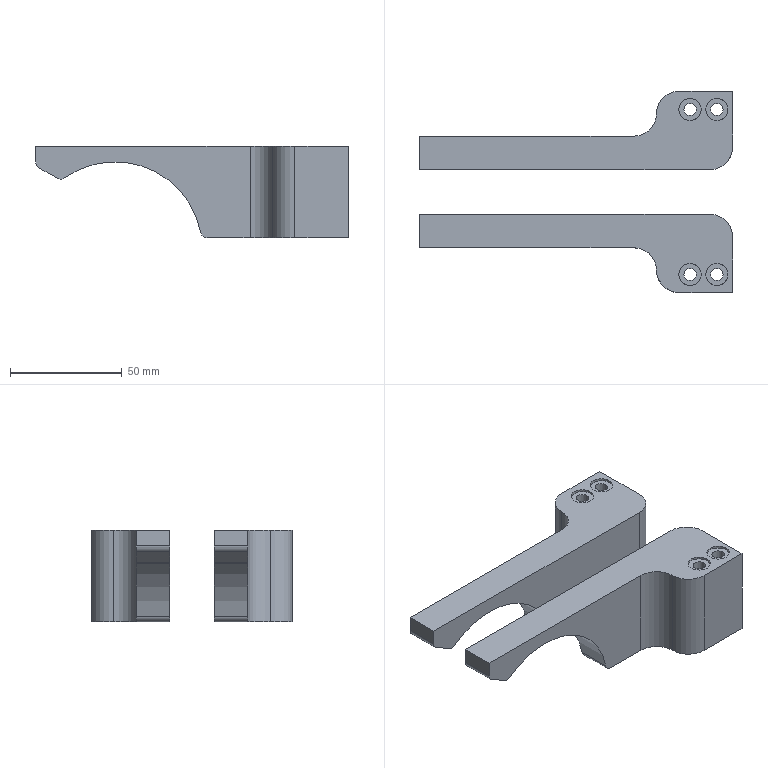NC program | NX | posted with a generic post | part box 140 x 90 x 41 mm
Lines 5568 to 5891 of 29499:
(ZLEVEL_PROFILE_COPY_COPY_COPY_1_COPY_COPY_COPY_COPY , TOOL : D12JING)
N11110 T11 M6
N11112 G54
N11114 G17 G0 G90 X-72.569 Y26.75 S9500 M3
N11116 G43 Z30. H11
N11118 Z-13.667
N11120 G94 G1 X-71.039 Y24.1 F1000.
N11122 G3 X-70. Y23.5 R1.2
N11124 G1 X60. F1200.
N11126 G2 X76. Y7.5 R16.
N11128 G1 Y-17.5
N11130 G2 X70. Y-23.5 R6.
N11132 G1 X46.
N11134 G2 X30. Y-7.5 R16.
N11136 G3 X26. Y-3.5 R4.
N11138 G1 X-70.
N11140 G2 X-76. Y2.5 R6.
N11142 G1 Y17.5
N11144 G2 X-70. Y23.5 R6.
N11146 G3 X-68.961 Y24.1 R1.2
N11148 G1 X-67.229 Y27.1
N11150 G0 X-72.569 Y26.75 Z-27.333
N11152 G1 X-71.039 Y24.1 F1000.
N11154 G3 X-70. Y23.5 R1.2
N11156 G1 X60. F1200.
N11158 G2 X76. Y7.5 R16.
N11160 G1 Y-17.5
N11162 G2 X70. Y-23.5 R6.
N11164 G1 X46.
N11166 G2 X30. Y-7.5 R16.
N11168 G3 X26. Y-3.5 R4.
N11170 G1 X-70.
N11172 G2 X-76. Y2.5 R6.
N11174 G1 Y17.5
N11176 G2 X-70. Y23.5 R6.
N11178 G3 X-68.961 Y24.1 R1.2
N11180 G1 X-67.229 Y27.1
N11182 G0 X-72.569 Y26.75 Z-41.
N11184 G1 X-71.039 Y24.1 F1000.
N11186 G3 X-70. Y23.5 R1.2
N11188 G1 X60. F1200.
N11190 G2 X76. Y7.5 R16.
N11192 G1 Y-17.5
N11194 G2 X70. Y-23.5 R6.
N11196 G1 X46.
N11198 G2 X30. Y-7.5 R16.
N11200 G3 X26. Y-3.5 R4.
N11202 G1 X-70.
N11204 G2 X-76. Y2.5 R6.
N11206 G1 Y17.5
N11208 G2 X-70. Y23.5 R6.
N11210 G3 X-68.961 Y24.1 R1.2
N11212 G1 X-67.229 Y27.1
N11214 G0 Z30.
(ZLEVEL_PROFILE_COPY , TOOL : D12JING)
N11216 X80.417 Y-9.398
N11218 Z-0.95
N11220 G1 X76.893 Y-9.377 F1650.
N11222 G3 X76.593 Y-9.297 R0.6
N11224 G1 X69.528 Y-9.3
N11226 X44.9
N11228 G3 X44.8 Y-9.4 R0.1
N11230 X44.9 Y-9.5 R0.1
N11232 G1 X69.528
N11234 X75.411 Y-9.498
N11236 X76.598 Y-9.503
N11238 G3 X76.899 Y-9.424 R0.6
N11240 G1 X80.417 Y-9.398
N11242 G0 Z-1.9
N11244 G1 X76.893 Y-9.377
N11246 G3 X76.593 Y-9.297 R0.6
N11248 G1 X69.528 Y-9.3
N11250 X44.9
N11252 G3 X44.8 Y-9.4 R0.1
N11254 X44.9 Y-9.5 R0.1
N11256 G1 X69.528
N11258 X70.369 Y-9.498
N11260 X75.411
N11262 X76.598 Y-9.503
N11264 G3 X76.899 Y-9.424 R0.6
N11266 G1 X80.417 Y-9.398
N11268 G0 Z-2.85
N11270 G1 X76.893 Y-9.377
N11272 G3 X76.593 Y-9.297 R0.6
N11274 G1 X69.528 Y-9.3
N11276 X44.9
N11278 G3 X44.8 Y-9.4 R0.1
N11280 X44.9 Y-9.5 R0.1
N11282 G1 X69.528
N11284 X70.369 Y-9.497
N11286 X75.411
N11288 X76.598 Y-9.503
N11290 G3 X76.899 Y-9.424 R0.6
N11292 G1 X80.417 Y-9.398
N11294 G0 X80.418 Y-9.399 Z-3.8
N11296 G1 X76.894 Y-9.376
N11298 G3 X76.593 Y-9.297 R0.6
N11300 G1 X75.411 Y-9.303
N11302 X70.369
N11304 X69.528 Y-9.3
N11306 X44.9
N11308 G3 X44.8 Y-9.4 R0.1
N11310 X44.9 Y-9.5 R0.1
N11312 G1 X69.528
N11314 X70.369 Y-9.497
N11316 X75.411
N11318 X76.598 Y-9.503
N11320 G3 X76.899 Y-9.424 R0.6
N11322 G1 X80.418 Y-9.399
N11324 G0 X80.419 Z-4.75
N11326 G1 X76.894 Y-9.376
N11328 G3 X76.593 Y-9.297 R0.6
N11330 G1 X75.411 Y-9.303
N11332 X70.369
N11334 X69.528 Y-9.3
N11336 X44.9
N11338 G3 X44.8 Y-9.4 R0.1
N11340 X44.9 Y-9.5 R0.1
N11342 G1 X69.528
N11344 X70.369 Y-9.497
N11346 X75.411
N11348 X76.598 Y-9.503
N11350 G3 X76.899 Y-9.424 R0.6
N11352 G1 X80.419 Y-9.399
N11354 G0 Z-5.7
N11356 G1 X76.894 Y-9.376
N11358 G3 X76.593 Y-9.298 R0.6
N11360 G1 X75.411 Y-9.303
N11362 X70.369
N11364 X69.528 Y-9.3
N11366 X44.9
N11368 G3 X44.8 Y-9.4 R0.1
N11370 X44.9 Y-9.5 R0.1
N11372 G1 X69.528
N11374 X70.369 Y-9.497
N11376 X75.411
N11378 X76.598 Y-9.502
N11380 G3 X76.899 Y-9.424 R0.6
N11382 G1 X80.419 Y-9.399
N11384 G0 Z-6.65
N11386 G1 X76.894 Y-9.377
N11388 G3 X76.593 Y-9.298 R0.6
N11390 G1 X75.411 Y-9.304
N11392 X70.369
N11394 X69.528 Y-9.3
N11396 X44.9
N11398 G3 X44.8 Y-9.4 R0.1
N11400 X44.9 Y-9.5 R0.1
N11402 G1 X69.528
N11404 X70.369 Y-9.496
N11406 X75.411
N11408 X76.598 Y-9.502
N11410 G3 X76.899 Y-9.423 R0.6
N11412 G1 X80.419 Y-9.399
N11414 G0 Z-7.6
N11416 G1 X76.894 Y-9.377
N11418 G3 X76.593 Y-9.298 R0.6
N11420 G1 X75.411 Y-9.304
N11422 X70.369
N11424 X69.528 Y-9.3
N11426 X44.9
N11428 G3 X44.8 Y-9.4 R0.1
N11430 X44.9 Y-9.5 R0.1
N11432 G1 X69.528
N11434 X70.369 Y-9.496
N11436 X75.411
N11438 X76.598 Y-9.502
N11440 G3 X76.899 Y-9.423 R0.6
N11442 G1 X80.419 Y-9.399
N11444 G0 Z-8.55
N11446 G1 X76.894 Y-9.377
N11448 G3 X76.593 Y-9.298 R0.6
N11450 G1 X75.411 Y-9.304
N11452 X70.369
N11454 X69.528 Y-9.3
N11456 X44.9
N11458 G3 X44.8 Y-9.4 R0.1
N11460 X44.9 Y-9.5 R0.1
N11462 G1 X69.528
N11464 X70.369 Y-9.496
N11466 X75.411
N11468 X76.598 Y-9.502
N11470 G3 X76.899 Y-9.423 R0.6
N11472 G1 X80.419 Y-9.399
N11474 G0 X80.42 Z-9.5
N11476 G1 X76.894 Y-9.377
N11478 G3 X76.593 Y-9.298 R0.6
N11480 G1 X75.411 Y-9.304
N11482 X70.369
N11484 X69.528 Y-9.3
N11486 X44.9
N11488 G3 X44.8 Y-9.4 R0.1
N11490 X44.9 Y-9.5 R0.1
N11492 G1 X69.528
N11494 X70.369 Y-9.496
N11496 X75.411
N11498 X76.598 Y-9.502
N11500 G3 X76.899 Y-9.423 R0.6
N11502 G1 X80.42 Y-9.399
N11504 G0 Z-10.45
N11506 G1 X76.894 Y-9.377
N11508 G3 X76.593 Y-9.298 R0.6
N11510 G1 X75.411 Y-9.305
N11512 X70.369
N11514 X69.528 Y-9.3
N11516 X44.9
N11518 G3 X44.8 Y-9.4 R0.1
N11520 X44.9 Y-9.5 R0.1
N11522 G1 X69.528
N11524 X70.369 Y-9.495
N11526 X75.411
N11528 X76.598 Y-9.502
N11530 G3 X76.899 Y-9.423 R0.6
N11532 G1 X80.42 Y-9.399
N11534 G0 Z-11.4
N11536 G1 X76.894 Y-9.377
N11538 G3 X76.593 Y-9.298 R0.6
N11540 G1 X75.411 Y-9.305
N11542 X70.369
N11544 X69.528 Y-9.3
N11546 X44.9
N11548 G3 X44.8 Y-9.4 R0.1
N11550 X44.9 Y-9.5 R0.1
N11552 G1 X69.528
N11554 X70.369 Y-9.495
N11556 X75.411
N11558 X76.598 Y-9.502
N11560 G3 X76.899 Y-9.423 R0.6
N11562 G1 X80.42 Y-9.399
N11564 G0 Z-12.35
N11566 G1 X76.894 Y-9.377
N11568 G3 X76.593 Y-9.299 R0.6
N11570 G1 X75.411 Y-9.305
N11572 X70.369
N11574 X69.528 Y-9.3
N11576 X44.9
N11578 G3 X44.8 Y-9.4 R0.1
N11580 X44.9 Y-9.5 R0.1
N11582 G1 X69.528
N11584 X70.369 Y-9.495
N11586 X75.411
N11588 X76.598 Y-9.501
N11590 G3 X76.899 Y-9.423 R0.6
N11592 G1 X80.42 Y-9.399
N11594 G0 X80.421 Z-13.3
N11596 G1 X76.894 Y-9.377
N11598 G3 X76.593 Y-9.299 R0.6
N11600 G1 X75.411 Y-9.305
N11602 X70.369
N11604 X69.528 Y-9.3
N11606 X44.9
N11608 G3 X44.8 Y-9.4 R0.1
N11610 X44.9 Y-9.5 R0.1
N11612 G1 X69.528
N11614 X70.369 Y-9.495
N11616 X75.411
N11618 X76.598 Y-9.501
N11620 G3 X76.899 Y-9.423 R0.6
N11622 G1 X80.421 Y-9.399
N11624 G0 Z-14.25
N11626 G1 X76.894 Y-9.377
N11628 G3 X76.593 Y-9.299 R0.6
N11630 G1 X75.411 Y-9.306
N11632 X70.369
N11634 X69.528 Y-9.3
N11636 X44.9
N11638 G3 X44.8 Y-9.4 R0.1
N11640 X44.9 Y-9.5 R0.1
N11642 G1 X69.528
N11644 X70.369 Y-9.494
N11646 X75.411
N11648 X76.598 Y-9.501
N11650 G3 X76.899 Y-9.423 R0.6
N11652 G1 X80.421 Y-9.399
N11654 G0 Z-15.2
N11656 G1 X76.894 Y-9.378
N11658 G3 X76.593 Y-9.299 R0.6
N11660 G1 X75.411 Y-9.306
N11662 X70.369
N11664 X69.528 Y-9.3
N11666 X44.9
N11668 G3 X44.8 Y-9.4 R0.1
N11670 X44.9 Y-9.5 R0.1
N11672 G1 X69.528
N11674 X70.369 Y-9.494
N11676 X75.411
N11678 X76.598 Y-9.501
N11680 G3 X76.899 Y-9.422 R0.6
N11682 G1 X80.421 Y-9.399
N11684 G0 Z30.
N11686 M5
(PLANAR_MILL_COPY , TOOL : D6A45)
N11688 T07 M6
N11690 G54
N11692 G17 G0 G90 X7.883 Y19.318 S9500 M3
N11694 G43 Z30. H7
N11696 Z0.
N11698 G94 G1 Z-1. F1250.
N11700 G3 X8.031 Y18.4 R1.
N11702 G1 X60.
N11704 G2 X70.9 Y7.5 R10.9
N11706 G1 Y-3.2
N11708 G2 X69.9 Y-4.2 R1.
N11710 G1 X44.9
N11712 G3 X39.7 Y-9.4 R5.2
N11714 X44.9 Y-14.6 R5.2
N11716 G1 X69.9
N11718 G2 X70.9 Y-15.6 R1.
N11720 G1 Y-17.4
N11722 G2 X69.9 Y-18.4 R1.
N11724 G1 X46.
N11726 G2 X35.1 Y-7.5 R10.9
N11728 G3 X26. Y1.6 R9.1
N11730 G1 X8.031
N11732 G3 X7.883 Y0.682 R1.
N11734 G1 Z0.
N11736 G0 Z30.
N11738 M5